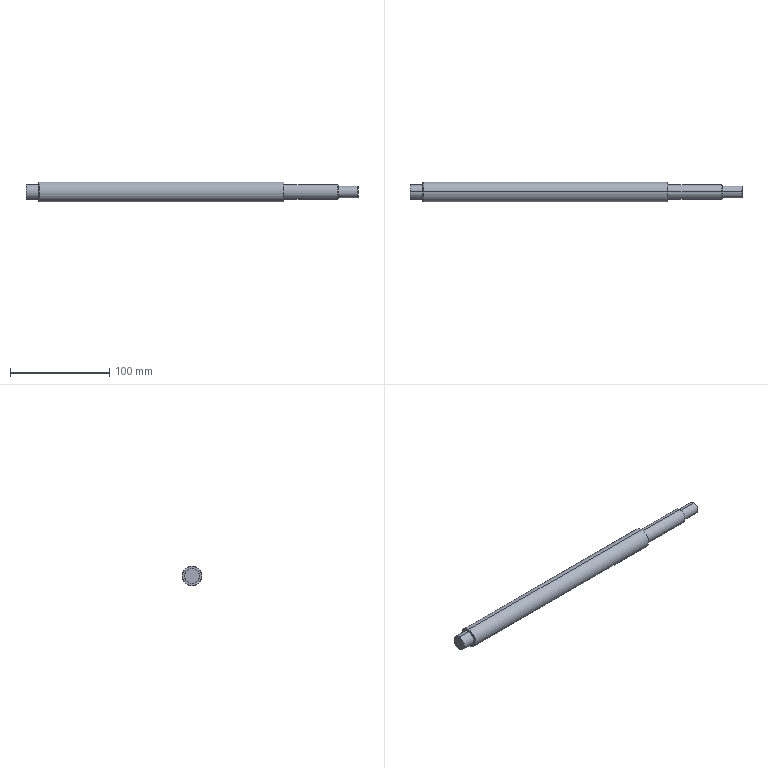Part | NX | features BREP 1 | 1 solid | 27 faces | box 335 x 20 x 20 mm | volume 91863 mm3 | cylinder 8 | torus 8 | cone 6 | plane 5 | commonest cylinder face diameters 15 x4 12 x2 20 x2
STEP:
#1=CARTESIAN_POINT('',(334.5,0.,6.));
#2=VERTEX_POINT('',#1);
#3=CARTESIAN_POINT('',(335.,0.,5.5));
#4=VERTEX_POINT('',#3);
#5=CARTESIAN_POINT('',(335.,0.,5.5));
#6=DIRECTION('',(-0.7071,0.,0.7071));
#7=VECTOR('',#6,1000.);
#8=LINE('',#5,#7);
#9=EDGE_CURVE('',#2,#4,#8,.F.);
#10=ORIENTED_EDGE('',*,*,#9,.T.);
#11=CARTESIAN_POINT('',(335.,0.,-5.5));
#12=VERTEX_POINT('',#11);
#13=CARTESIAN_POINT('',(335.,0.,0.));
#14=DIRECTION('',(1.,0.,0.));
#15=DIRECTION('',(0.,0.,-1.));
#16=AXIS2_PLACEMENT_3D('',#13,#14,#15);
#17=CIRCLE('',#16,5.5);
#18=EDGE_CURVE('',#12,#4,#17,.T.);
#19=ORIENTED_EDGE('',*,*,#18,.F.);
#20=CARTESIAN_POINT('',(334.5,0.,-6.));
#21=VERTEX_POINT('',#20);
#22=CARTESIAN_POINT('',(335.,0.,-5.5));
#23=DIRECTION('',(-0.7071,0.,-0.7071));
#24=VECTOR('',#23,1000.);
#25=LINE('',#22,#24);
#26=EDGE_CURVE('',#21,#12,#25,.F.);
#27=ORIENTED_EDGE('',*,*,#26,.F.);
#28=CARTESIAN_POINT('',(334.5,0.,0.));
#29=DIRECTION('',(1.,0.,0.));
#30=DIRECTION('',(0.,0.,-1.));
#31=AXIS2_PLACEMENT_3D('',#28,#29,#30);
#32=CIRCLE('',#31,6.);
#33=EDGE_CURVE('',#21,#2,#32,.T.);
#34=ORIENTED_EDGE('',*,*,#33,.T.);
#35=EDGE_LOOP('',(#10,#19,#27,#34));
#36=FACE_BOUND('',#35,.T.);
#37=CARTESIAN_POINT('',(334.75,0.,0.));
#38=DIRECTION('',(-1.,0.,0.));
#39=DIRECTION('',(0.,0.,1.));
#40=AXIS2_PLACEMENT_3D('',#37,#38,#39);
#41=CONICAL_SURFACE('',#40,5.75,0.7854);
#42=ADVANCED_FACE('',(#36),#41,.T.);
#43=CARTESIAN_POINT('',(315.,0.,6.));
#44=VERTEX_POINT('',#43);
#45=CARTESIAN_POINT('',(334.5,0.,6.));
#46=DIRECTION('',(-1.,0.,0.));
#47=VECTOR('',#46,1000.);
#48=LINE('',#45,#47);
#49=EDGE_CURVE('',#44,#2,#48,.F.);
#50=ORIENTED_EDGE('',*,*,#49,.T.);
#51=ORIENTED_EDGE('',*,*,#33,.F.);
#52=CARTESIAN_POINT('',(315.,0.,-6.));
#53=VERTEX_POINT('',#52);
#54=CARTESIAN_POINT('',(334.5,0.,-6.));
#55=DIRECTION('',(-1.,0.,0.));
#56=VECTOR('',#55,1000.);
#57=LINE('',#54,#56);
#58=EDGE_CURVE('',#53,#21,#57,.F.);
#59=ORIENTED_EDGE('',*,*,#58,.F.);
#60=CARTESIAN_POINT('',(315.,0.,0.));
#61=DIRECTION('',(-1.,0.,0.));
#62=DIRECTION('',(0.,0.,1.));
#63=AXIS2_PLACEMENT_3D('',#60,#61,#62);
#64=CIRCLE('',#63,6.);
#65=EDGE_CURVE('',#44,#53,#64,.T.);
#66=ORIENTED_EDGE('',*,*,#65,.F.);
#67=EDGE_LOOP('',(#50,#51,#59,#66));
#68=FACE_BOUND('',#67,.T.);
#69=CARTESIAN_POINT('',(335.,0.,0.));
#70=DIRECTION('',(-1.,0.,0.));
#71=DIRECTION('',(0.,0.,-1.));
#72=AXIS2_PLACEMENT_3D('',#69,#70,#71);
#73=CYLINDRICAL_SURFACE('',#72,6.);
#74=ADVANCED_FACE('',(#68),#73,.T.);
#75=CARTESIAN_POINT('',(315.,0.,7.));
#76=VERTEX_POINT('',#75);
#77=CARTESIAN_POINT('',(315.,0.,-7.));
#78=VERTEX_POINT('',#77);
#79=CARTESIAN_POINT('',(315.,0.,0.));
#80=DIRECTION('',(1.,0.,0.));
#81=DIRECTION('',(0.,0.,1.));
#82=AXIS2_PLACEMENT_3D('',#79,#80,#81);
#83=CIRCLE('',#82,7.);
#84=EDGE_CURVE('',#76,#78,#83,.T.);
#85=ORIENTED_EDGE('',*,*,#84,.T.);
#86=CARTESIAN_POINT('',(315.,0.,0.));
#87=DIRECTION('',(1.,0.,0.));
#88=DIRECTION('',(0.,0.,-1.));
#89=AXIS2_PLACEMENT_3D('',#86,#87,#88);
#90=CIRCLE('',#89,7.);
#91=EDGE_CURVE('',#78,#76,#90,.T.);
#92=ORIENTED_EDGE('',*,*,#91,.T.);
#93=EDGE_LOOP('',(#85,#92));
#94=FACE_BOUND('',#93,.T.);
#95=ORIENTED_EDGE('',*,*,#65,.T.);
#96=CARTESIAN_POINT('',(315.,0.,0.));
#97=DIRECTION('',(-1.,0.,0.));
#98=DIRECTION('',(0.,0.,-1.));
#99=AXIS2_PLACEMENT_3D('',#96,#97,#98);
#100=CIRCLE('',#99,6.);
#101=EDGE_CURVE('',#53,#44,#100,.T.);
#102=ORIENTED_EDGE('',*,*,#101,.T.);
#103=EDGE_LOOP('',(#95,#102));
#104=FACE_BOUND('',#103,.T.);
#105=CARTESIAN_POINT('',(315.,7.,0.));
#106=DIRECTION('',(-1.,0.,0.));
#107=DIRECTION('',(0.,0.,1.));
#108=AXIS2_PLACEMENT_3D('',#105,#106,#107);
#109=PLANE('',#108);
#110=ADVANCED_FACE('',(#94,#104),#109,.F.);
#111=CARTESIAN_POINT('',(314.5,0.,7.5));
#112=VERTEX_POINT('',#111);
#113=CARTESIAN_POINT('',(315.,0.,7.));
#114=DIRECTION('',(-0.7071,0.,0.7071));
#115=VECTOR('',#114,1000.);
#116=LINE('',#113,#115);
#117=EDGE_CURVE('',#112,#76,#116,.F.);
#118=ORIENTED_EDGE('',*,*,#117,.T.);
#119=ORIENTED_EDGE('',*,*,#91,.F.);
#120=CARTESIAN_POINT('',(314.5,0.,-7.5));
#121=VERTEX_POINT('',#120);
#122=CARTESIAN_POINT('',(315.,0.,-7.));
#123=DIRECTION('',(-0.7071,0.,-0.7071));
#124=VECTOR('',#123,1000.);
#125=LINE('',#122,#124);
#126=EDGE_CURVE('',#121,#78,#125,.F.);
#127=ORIENTED_EDGE('',*,*,#126,.F.);
#128=CARTESIAN_POINT('',(314.5,0.,0.));
#129=DIRECTION('',(1.,0.,0.));
#130=DIRECTION('',(0.,0.,-1.));
#131=AXIS2_PLACEMENT_3D('',#128,#129,#130);
#132=CIRCLE('',#131,7.5);
#133=EDGE_CURVE('',#121,#112,#132,.T.);
#134=ORIENTED_EDGE('',*,*,#133,.T.);
#135=EDGE_LOOP('',(#118,#119,#127,#134));
#136=FACE_BOUND('',#135,.T.);
#137=CARTESIAN_POINT('',(314.75,0.,0.));
#138=DIRECTION('',(-1.,0.,0.));
#139=DIRECTION('',(0.,0.,1.));
#140=AXIS2_PLACEMENT_3D('',#137,#138,#139);
#141=CONICAL_SURFACE('',#140,7.25,0.7854);
#142=ADVANCED_FACE('',(#136),#141,.T.);
#143=CARTESIAN_POINT('',(260.1,0.,7.5));
#144=VERTEX_POINT('',#143);
#145=CARTESIAN_POINT('',(314.5,0.,7.5));
#146=DIRECTION('',(-1.,0.,0.));
#147=VECTOR('',#146,1000.);
#148=LINE('',#145,#147);
#149=EDGE_CURVE('',#144,#112,#148,.F.);
#150=ORIENTED_EDGE('',*,*,#149,.T.);
#151=ORIENTED_EDGE('',*,*,#133,.F.);
#152=CARTESIAN_POINT('',(260.1,0.,-7.5));
#153=VERTEX_POINT('',#152);
#154=CARTESIAN_POINT('',(314.5,0.,-7.5));
#155=DIRECTION('',(-1.,0.,0.));
#156=VECTOR('',#155,1000.);
#157=LINE('',#154,#156);
#158=EDGE_CURVE('',#153,#121,#157,.F.);
#159=ORIENTED_EDGE('',*,*,#158,.F.);
#160=CARTESIAN_POINT('',(260.1,0.,0.));
#161=DIRECTION('',(-1.,0.,0.));
#162=DIRECTION('',(0.,0.,1.));
#163=AXIS2_PLACEMENT_3D('',#160,#161,#162);
#164=CIRCLE('',#163,7.5);
#165=EDGE_CURVE('',#144,#153,#164,.T.);
#166=ORIENTED_EDGE('',*,*,#165,.F.);
#167=EDGE_LOOP('',(#150,#151,#159,#166));
#168=FACE_BOUND('',#167,.T.);
#169=CARTESIAN_POINT('',(335.,0.,0.));
#170=DIRECTION('',(-1.,0.,0.));
#171=DIRECTION('',(0.,0.,-1.));
#172=AXIS2_PLACEMENT_3D('',#169,#170,#171);
#173=CYLINDRICAL_SURFACE('',#172,7.5);
#174=ADVANCED_FACE('',(#168),#173,.T.);
#175=CARTESIAN_POINT('',(260.029,0.,-7.529));
#176=VERTEX_POINT('',#175);
#177=CARTESIAN_POINT('',(260.1,0.,-7.6));
#178=DIRECTION('',(0.,-1.,0.));
#179=DIRECTION('',(0.,0.,1.));
#180=AXIS2_PLACEMENT_3D('',#177,#178,#179);
#181=CIRCLE('',#180,0.1);
#182=EDGE_CURVE('',#153,#176,#181,.T.);
#183=ORIENTED_EDGE('',*,*,#182,.T.);
#184=CARTESIAN_POINT('',(260.029,0.,7.529));
#185=VERTEX_POINT('',#184);
#186=CARTESIAN_POINT('',(260.029,0.,0.));
#187=DIRECTION('',(1.,0.,0.));
#188=DIRECTION('',(0.,0.,-1.));
#189=AXIS2_PLACEMENT_3D('',#186,#187,#188);
#190=CIRCLE('',#189,7.529);
#191=EDGE_CURVE('',#176,#185,#190,.T.);
#192=ORIENTED_EDGE('',*,*,#191,.T.);
#193=CARTESIAN_POINT('',(260.1,0.,7.6));
#194=DIRECTION('',(0.,1.,0.));
#195=DIRECTION('',(0.,0.,-1.));
#196=AXIS2_PLACEMENT_3D('',#193,#194,#195);
#197=CIRCLE('',#196,0.1);
#198=EDGE_CURVE('',#144,#185,#197,.T.);
#199=ORIENTED_EDGE('',*,*,#198,.F.);
#200=ORIENTED_EDGE('',*,*,#165,.T.);
#201=EDGE_LOOP('',(#183,#192,#199,#200));
#202=FACE_BOUND('',#201,.T.);
#203=CARTESIAN_POINT('',(260.1,0.,0.));
#204=DIRECTION('',(1.,0.,0.));
#205=DIRECTION('',(0.,0.,-1.));
#206=AXIS2_PLACEMENT_3D('',#203,#204,#205);
#207=TOROIDAL_SURFACE('',#206,7.6,0.1);
#208=ADVANCED_FACE('',(#202),#207,.F.);
#209=ORIENTED_EDGE('',*,*,#198,.T.);
#210=CARTESIAN_POINT('',(260.029,0.,0.));
#211=DIRECTION('',(1.,0.,0.));
#212=DIRECTION('',(0.,0.,1.));
#213=AXIS2_PLACEMENT_3D('',#210,#211,#212);
#214=CIRCLE('',#213,7.529);
#215=EDGE_CURVE('',#185,#176,#214,.T.);
#216=ORIENTED_EDGE('',*,*,#215,.T.);
#217=ORIENTED_EDGE('',*,*,#182,.F.);
#218=CARTESIAN_POINT('',(260.1,0.,0.));
#219=DIRECTION('',(-1.,0.,0.));
#220=DIRECTION('',(0.,0.,-1.));
#221=AXIS2_PLACEMENT_3D('',#218,#219,#220);
#222=CIRCLE('',#221,7.5);
#223=EDGE_CURVE('',#153,#144,#222,.T.);
#224=ORIENTED_EDGE('',*,*,#223,.T.);
#225=EDGE_LOOP('',(#209,#216,#217,#224));
#226=FACE_BOUND('',#225,.T.);
#227=CARTESIAN_POINT('',(260.1,0.,0.));
#228=DIRECTION('',(1.,0.,0.));
#229=DIRECTION('',(0.,0.,-1.));
#230=AXIS2_PLACEMENT_3D('',#227,#228,#229);
#231=TOROIDAL_SURFACE('',#230,7.6,0.1);
#232=ADVANCED_FACE('',(#226),#231,.F.);
#233=ORIENTED_EDGE('',*,*,#158,.T.);
#234=CARTESIAN_POINT('',(314.5,0.,0.));
#235=DIRECTION('',(1.,0.,0.));
#236=DIRECTION('',(0.,0.,1.));
#237=AXIS2_PLACEMENT_3D('',#234,#235,#236);
#238=CIRCLE('',#237,7.5);
#239=EDGE_CURVE('',#112,#121,#238,.T.);
#240=ORIENTED_EDGE('',*,*,#239,.F.);
#241=ORIENTED_EDGE('',*,*,#149,.F.);
#242=ORIENTED_EDGE('',*,*,#223,.F.);
#243=EDGE_LOOP('',(#233,#240,#241,#242));
#244=FACE_BOUND('',#243,.T.);
#245=CARTESIAN_POINT('',(335.,0.,0.));
#246=DIRECTION('',(-1.,0.,0.));
#247=DIRECTION('',(0.,0.,-1.));
#248=AXIS2_PLACEMENT_3D('',#245,#246,#247);
#249=CYLINDRICAL_SURFACE('',#248,7.5);
#250=ADVANCED_FACE('',(#244),#249,.T.);
#251=ORIENTED_EDGE('',*,*,#126,.T.);
#252=ORIENTED_EDGE('',*,*,#84,.F.);
#253=ORIENTED_EDGE('',*,*,#117,.F.);
#254=ORIENTED_EDGE('',*,*,#239,.T.);
#255=EDGE_LOOP('',(#251,#252,#253,#254));
#256=FACE_BOUND('',#255,.T.);
#257=CARTESIAN_POINT('',(314.75,0.,0.));
#258=DIRECTION('',(-1.,0.,0.));
#259=DIRECTION('',(0.,0.,1.));
#260=AXIS2_PLACEMENT_3D('',#257,#258,#259);
#261=CONICAL_SURFACE('',#260,7.25,0.7854);
#262=ADVANCED_FACE('',(#256),#261,.T.);
#263=CARTESIAN_POINT('',(260.,0.,-7.6));
#264=VERTEX_POINT('',#263);
#265=CARTESIAN_POINT('',(260.1,0.,-7.6));
#266=DIRECTION('',(0.,-1.,0.));
#267=DIRECTION('',(-0.7071,0.,0.7071));
#268=AXIS2_PLACEMENT_3D('',#265,#266,#267);
#269=CIRCLE('',#268,0.1);
#270=EDGE_CURVE('',#176,#264,#269,.T.);
#271=ORIENTED_EDGE('',*,*,#270,.F.);
#272=ORIENTED_EDGE('',*,*,#215,.F.);
#273=CARTESIAN_POINT('',(260.,0.,7.6));
#274=VERTEX_POINT('',#273);
#275=CARTESIAN_POINT('',(260.1,0.,7.6));
#276=DIRECTION('',(0.,1.,0.));
#277=DIRECTION('',(-0.7071,0.,-0.7071));
#278=AXIS2_PLACEMENT_3D('',#275,#276,#277);
#279=CIRCLE('',#278,0.1);
#280=EDGE_CURVE('',#185,#274,#279,.T.);
#281=ORIENTED_EDGE('',*,*,#280,.T.);
#282=CARTESIAN_POINT('',(260.,0.,0.));
#283=DIRECTION('',(-1.,0.,0.));
#284=DIRECTION('',(0.,0.,-1.));
#285=AXIS2_PLACEMENT_3D('',#282,#283,#284);
#286=CIRCLE('',#285,7.6);
#287=EDGE_CURVE('',#264,#274,#286,.T.);
#288=ORIENTED_EDGE('',*,*,#287,.F.);
#289=EDGE_LOOP('',(#271,#272,#281,#288));
#290=FACE_BOUND('',#289,.T.);
#291=CARTESIAN_POINT('',(260.1,0.,0.));
#292=DIRECTION('',(1.,0.,0.));
#293=DIRECTION('',(0.,0.,-1.));
#294=AXIS2_PLACEMENT_3D('',#291,#292,#293);
#295=TOROIDAL_SURFACE('',#294,7.6,0.1);
#296=ADVANCED_FACE('',(#290),#295,.F.);
#297=CARTESIAN_POINT('',(260.,0.,10.));
#298=VERTEX_POINT('',#297);
#299=CARTESIAN_POINT('',(260.,0.,-10.));
#300=VERTEX_POINT('',#299);
#301=CARTESIAN_POINT('',(260.,0.,0.));
#302=DIRECTION('',(1.,0.,0.));
#303=DIRECTION('',(0.,0.,1.));
#304=AXIS2_PLACEMENT_3D('',#301,#302,#303);
#305=CIRCLE('',#304,10.);
#306=EDGE_CURVE('',#298,#300,#305,.T.);
#307=ORIENTED_EDGE('',*,*,#306,.T.);
#308=CARTESIAN_POINT('',(260.,0.,0.));
#309=DIRECTION('',(1.,0.,0.));
#310=DIRECTION('',(0.,0.,-1.));
#311=AXIS2_PLACEMENT_3D('',#308,#309,#310);
#312=CIRCLE('',#311,10.);
#313=EDGE_CURVE('',#300,#298,#312,.T.);
#314=ORIENTED_EDGE('',*,*,#313,.T.);
#315=EDGE_LOOP('',(#307,#314));
#316=FACE_BOUND('',#315,.T.);
#317=CARTESIAN_POINT('',(260.,0.,0.));
#318=DIRECTION('',(-1.,0.,0.));
#319=DIRECTION('',(0.,0.,1.));
#320=AXIS2_PLACEMENT_3D('',#317,#318,#319);
#321=CIRCLE('',#320,7.6);
#322=EDGE_CURVE('',#274,#264,#321,.T.);
#323=ORIENTED_EDGE('',*,*,#322,.T.);
#324=ORIENTED_EDGE('',*,*,#287,.T.);
#325=EDGE_LOOP('',(#323,#324));
#326=FACE_BOUND('',#325,.T.);
#327=CARTESIAN_POINT('',(260.,10.,0.));
#328=DIRECTION('',(-1.,0.,0.));
#329=DIRECTION('',(0.,0.,1.));
#330=AXIS2_PLACEMENT_3D('',#327,#328,#329);
#331=PLANE('',#330);
#332=ADVANCED_FACE('',(#316,#326),#331,.F.);
#333=CARTESIAN_POINT('',(13.3,0.,10.));
#334=VERTEX_POINT('',#333);
#335=CARTESIAN_POINT('',(260.,0.,10.));
#336=DIRECTION('',(-1.,0.,0.));
#337=VECTOR('',#336,1000.);
#338=LINE('',#335,#337);
#339=EDGE_CURVE('',#334,#298,#338,.F.);
#340=ORIENTED_EDGE('',*,*,#339,.T.);
#341=ORIENTED_EDGE('',*,*,#313,.F.);
#342=CARTESIAN_POINT('',(13.3,0.,-10.));
#343=VERTEX_POINT('',#342);
#344=CARTESIAN_POINT('',(260.,0.,-10.));
#345=DIRECTION('',(-1.,0.,0.));
#346=VECTOR('',#345,1000.);
#347=LINE('',#344,#346);
#348=EDGE_CURVE('',#343,#300,#347,.F.);
#349=ORIENTED_EDGE('',*,*,#348,.F.);
#350=CARTESIAN_POINT('',(13.3,0.,0.));
#351=DIRECTION('',(-1.,0.,0.));
#352=DIRECTION('',(0.,0.,1.));
#353=AXIS2_PLACEMENT_3D('',#350,#351,#352);
#354=CIRCLE('',#353,10.);
#355=EDGE_CURVE('',#334,#343,#354,.T.);
#356=ORIENTED_EDGE('',*,*,#355,.F.);
#357=EDGE_LOOP('',(#340,#341,#349,#356));
#358=FACE_BOUND('',#357,.T.);
#359=CARTESIAN_POINT('',(335.,0.,0.));
#360=DIRECTION('',(-1.,0.,0.));
#361=DIRECTION('',(0.,0.,-1.));
#362=AXIS2_PLACEMENT_3D('',#359,#360,#361);
#363=CYLINDRICAL_SURFACE('',#362,10.);
#364=ADVANCED_FACE('',(#358),#363,.T.);
#365=CARTESIAN_POINT('',(13.,0.,-9.7));
#366=VERTEX_POINT('',#365);
#367=CARTESIAN_POINT('',(13.,0.,-9.7));
#368=DIRECTION('',(0.7071,0.,-0.7071));
#369=VECTOR('',#368,1000.);
#370=LINE('',#367,#369);
#371=EDGE_CURVE('',#366,#343,#370,.T.);
#372=ORIENTED_EDGE('',*,*,#371,.F.);
#373=CARTESIAN_POINT('',(13.,0.,9.7));
#374=VERTEX_POINT('',#373);
#375=CARTESIAN_POINT('',(13.,0.,0.));
#376=DIRECTION('',(-1.,0.,0.));
#377=DIRECTION('',(0.,0.,1.));
#378=AXIS2_PLACEMENT_3D('',#375,#376,#377);
#379=CIRCLE('',#378,9.7);
#380=EDGE_CURVE('',#374,#366,#379,.T.);
#381=ORIENTED_EDGE('',*,*,#380,.F.);
#382=CARTESIAN_POINT('',(13.,0.,9.7));
#383=DIRECTION('',(0.7071,0.,0.7071));
#384=VECTOR('',#383,1000.);
#385=LINE('',#382,#384);
#386=EDGE_CURVE('',#374,#334,#385,.T.);
#387=ORIENTED_EDGE('',*,*,#386,.T.);
#388=ORIENTED_EDGE('',*,*,#355,.T.);
#389=EDGE_LOOP('',(#372,#381,#387,#388));
#390=FACE_BOUND('',#389,.T.);
#391=CARTESIAN_POINT('',(13.15,0.,0.));
#392=DIRECTION('',(1.,0.,0.));
#393=DIRECTION('',(0.,0.,-1.));
#394=AXIS2_PLACEMENT_3D('',#391,#392,#393);
#395=CONICAL_SURFACE('',#394,9.85,0.7854);
#396=ADVANCED_FACE('',(#390),#395,.T.);
#397=ORIENTED_EDGE('',*,*,#386,.F.);
#398=CARTESIAN_POINT('',(13.,0.,0.));
#399=DIRECTION('',(-1.,0.,0.));
#400=DIRECTION('',(0.,0.,-1.));
#401=AXIS2_PLACEMENT_3D('',#398,#399,#400);
#402=CIRCLE('',#401,9.7);
#403=EDGE_CURVE('',#366,#374,#402,.T.);
#404=ORIENTED_EDGE('',*,*,#403,.F.);
#405=ORIENTED_EDGE('',*,*,#371,.T.);
#406=CARTESIAN_POINT('',(13.3,0.,0.));
#407=DIRECTION('',(-1.,0.,0.));
#408=DIRECTION('',(0.,0.,-1.));
#409=AXIS2_PLACEMENT_3D('',#406,#407,#408);
#410=CIRCLE('',#409,10.);
#411=EDGE_CURVE('',#343,#334,#410,.T.);
#412=ORIENTED_EDGE('',*,*,#411,.T.);
#413=EDGE_LOOP('',(#397,#404,#405,#412));
#414=FACE_BOUND('',#413,.T.);
#415=CARTESIAN_POINT('',(13.15,0.,0.));
#416=DIRECTION('',(1.,0.,0.));
#417=DIRECTION('',(0.,0.,-1.));
#418=AXIS2_PLACEMENT_3D('',#415,#416,#417);
#419=CONICAL_SURFACE('',#418,9.85,0.7854);
#420=ADVANCED_FACE('',(#414),#419,.T.);
#421=ORIENTED_EDGE('',*,*,#348,.T.);
#422=ORIENTED_EDGE('',*,*,#306,.F.);
#423=ORIENTED_EDGE('',*,*,#339,.F.);
#424=ORIENTED_EDGE('',*,*,#411,.F.);
#425=EDGE_LOOP('',(#421,#422,#423,#424));
#426=FACE_BOUND('',#425,.T.);
#427=CARTESIAN_POINT('',(335.,0.,0.));
#428=DIRECTION('',(-1.,0.,0.));
#429=DIRECTION('',(0.,0.,-1.));
#430=AXIS2_PLACEMENT_3D('',#427,#428,#429);
#431=CYLINDRICAL_SURFACE('',#430,10.);
#432=ADVANCED_FACE('',(#426),#431,.T.);
#433=ORIENTED_EDGE('',*,*,#380,.T.);
#434=ORIENTED_EDGE('',*,*,#403,.T.);
#435=EDGE_LOOP('',(#433,#434));
#436=FACE_BOUND('',#435,.T.);
#437=CARTESIAN_POINT('',(13.,0.,7.6));
#438=VERTEX_POINT('',#437);
#439=CARTESIAN_POINT('',(13.,0.,-7.6));
#440=VERTEX_POINT('',#439);
#441=CARTESIAN_POINT('',(13.,0.,0.));
#442=DIRECTION('',(1.,0.,0.));
#443=DIRECTION('',(0.,0.,1.));
#444=AXIS2_PLACEMENT_3D('',#441,#442,#443);
#445=CIRCLE('',#444,7.6);
#446=EDGE_CURVE('',#438,#440,#445,.T.);
#447=ORIENTED_EDGE('',*,*,#446,.T.);
#448=CARTESIAN_POINT('',(13.,0.,0.));
#449=DIRECTION('',(1.,0.,0.));
#450=DIRECTION('',(0.,0.,-1.));
#451=AXIS2_PLACEMENT_3D('',#448,#449,#450);
#452=CIRCLE('',#451,7.6);
#453=EDGE_CURVE('',#440,#438,#452,.T.);
#454=ORIENTED_EDGE('',*,*,#453,.T.);
#455=EDGE_LOOP('',(#447,#454));
#456=FACE_BOUND('',#455,.T.);
#457=CARTESIAN_POINT('',(13.,7.6,0.));
#458=DIRECTION('',(1.,0.,0.));
#459=DIRECTION('',(0.,1.,0.));
#460=AXIS2_PLACEMENT_3D('',#457,#458,#459);
#461=PLANE('',#460);
#462=ADVANCED_FACE('',(#436,#456),#461,.F.);
#463=CARTESIAN_POINT('',(12.971,0.,-7.529));
#464=VERTEX_POINT('',#463);
#465=CARTESIAN_POINT('',(12.9,0.,-7.6));
#466=DIRECTION('',(0.,-1.,0.));
#467=DIRECTION('',(1.,0.,0.));
#468=AXIS2_PLACEMENT_3D('',#465,#466,#467);
#469=CIRCLE('',#468,0.1);
#470=EDGE_CURVE('',#440,#464,#469,.T.);
#471=ORIENTED_EDGE('',*,*,#470,.T.);
#472=CARTESIAN_POINT('',(12.971,0.,7.529));
#473=VERTEX_POINT('',#472);
#474=CARTESIAN_POINT('',(12.971,0.,0.));
#475=DIRECTION('',(1.,0.,0.));
#476=DIRECTION('',(0.,0.,-1.));
#477=AXIS2_PLACEMENT_3D('',#474,#475,#476);
#478=CIRCLE('',#477,7.529);
#479=EDGE_CURVE('',#464,#473,#478,.T.);
#480=ORIENTED_EDGE('',*,*,#479,.T.);
#481=CARTESIAN_POINT('',(12.9,0.,7.6));
#482=DIRECTION('',(0.,1.,0.));
#483=DIRECTION('',(1.,0.,0.));
#484=AXIS2_PLACEMENT_3D('',#481,#482,#483);
#485=CIRCLE('',#484,0.1);
#486=EDGE_CURVE('',#438,#473,#485,.T.);
#487=ORIENTED_EDGE('',*,*,#486,.F.);
#488=ORIENTED_EDGE('',*,*,#453,.F.);
#489=EDGE_LOOP('',(#471,#480,#487,#488));
#490=FACE_BOUND('',#489,.T.);
#491=CARTESIAN_POINT('',(12.9,0.,0.));
#492=DIRECTION('',(1.,0.,0.));
#493=DIRECTION('',(0.,0.,-1.));
#494=AXIS2_PLACEMENT_3D('',#491,#492,#493);
#495=TOROIDAL_SURFACE('',#494,7.6,0.1);
#496=ADVANCED_FACE('',(#490),#495,.F.);
#497=ORIENTED_EDGE('',*,*,#486,.T.);
#498=CARTESIAN_POINT('',(12.971,0.,0.));
#499=DIRECTION('',(1.,0.,0.));
#500=DIRECTION('',(0.,0.,1.));
#501=AXIS2_PLACEMENT_3D('',#498,#499,#500);
#502=CIRCLE('',#501,7.529);
#503=EDGE_CURVE('',#473,#464,#502,.T.);
#504=ORIENTED_EDGE('',*,*,#503,.T.);
#505=ORIENTED_EDGE('',*,*,#470,.F.);
#506=ORIENTED_EDGE('',*,*,#446,.F.);
#507=EDGE_LOOP('',(#497,#504,#505,#506));
#508=FACE_BOUND('',#507,.T.);
#509=CARTESIAN_POINT('',(12.9,0.,0.));
#510=DIRECTION('',(1.,0.,0.));
#511=DIRECTION('',(0.,0.,-1.));
#512=AXIS2_PLACEMENT_3D('',#509,#510,#511);
#513=TOROIDAL_SURFACE('',#512,7.6,0.1);
#514=ADVANCED_FACE('',(#508),#513,.F.);
#515=CARTESIAN_POINT('',(12.9,0.,-7.5));
#516=VERTEX_POINT('',#515);
#517=CARTESIAN_POINT('',(12.9,0.,-7.6));
#518=DIRECTION('',(0.,-1.,0.));
#519=DIRECTION('',(0.7071,0.,0.7071));
#520=AXIS2_PLACEMENT_3D('',#517,#518,#519);
#521=CIRCLE('',#520,0.1);
#522=EDGE_CURVE('',#464,#516,#521,.T.);
#523=ORIENTED_EDGE('',*,*,#522,.F.);
#524=ORIENTED_EDGE('',*,*,#503,.F.);
#525=CARTESIAN_POINT('',(12.9,0.,7.5));
#526=VERTEX_POINT('',#525);
#527=CARTESIAN_POINT('',(12.9,0.,7.6));
#528=DIRECTION('',(0.,1.,0.));
#529=DIRECTION('',(0.7071,0.,-0.7071));
#530=AXIS2_PLACEMENT_3D('',#527,#528,#529);
#531=CIRCLE('',#530,0.1);
#532=EDGE_CURVE('',#473,#526,#531,.T.);
#533=ORIENTED_EDGE('',*,*,#532,.T.);
#534=CARTESIAN_POINT('',(12.9,0.,0.));
#535=DIRECTION('',(1.,0.,0.));
#536=DIRECTION('',(0.,0.,1.));
#537=AXIS2_PLACEMENT_3D('',#534,#535,#536);
#538=CIRCLE('',#537,7.5);
#539=EDGE_CURVE('',#526,#516,#538,.T.);
#540=ORIENTED_EDGE('',*,*,#539,.T.);
#541=EDGE_LOOP('',(#523,#524,#533,#540));
#542=FACE_BOUND('',#541,.T.);
#543=CARTESIAN_POINT('',(12.9,0.,0.));
#544=DIRECTION('',(1.,0.,0.));
#545=DIRECTION('',(0.,0.,-1.));
#546=AXIS2_PLACEMENT_3D('',#543,#544,#545);
#547=TOROIDAL_SURFACE('',#546,7.6,0.1);
#548=ADVANCED_FACE('',(#542),#547,.F.);
#549=CARTESIAN_POINT('',(0.,0.,-7.5));
#550=VERTEX_POINT('',#549);
#551=CARTESIAN_POINT('',(12.9,0.,-7.5));
#552=DIRECTION('',(-1.,0.,0.));
#553=VECTOR('',#552,1000.);
#554=LINE('',#551,#553);
#555=EDGE_CURVE('',#516,#550,#554,.T.);
#556=ORIENTED_EDGE('',*,*,#555,.F.);
#557=ORIENTED_EDGE('',*,*,#539,.F.);
#558=CARTESIAN_POINT('',(0.,0.,7.5));
#559=VERTEX_POINT('',#558);
#560=CARTESIAN_POINT('',(12.9,0.,7.5));
#561=DIRECTION('',(-1.,0.,0.));
#562=VECTOR('',#561,1000.);
#563=LINE('',#560,#562);
#564=EDGE_CURVE('',#526,#559,#563,.T.);
#565=ORIENTED_EDGE('',*,*,#564,.T.);
#566=CARTESIAN_POINT('',(0.,0.,0.));
#567=DIRECTION('',(-1.,0.,0.));
#568=DIRECTION('',(0.,0.,-1.));
#569=AXIS2_PLACEMENT_3D('',#566,#567,#568);
#570=CIRCLE('',#569,7.5);
#571=EDGE_CURVE('',#550,#559,#570,.T.);
#572=ORIENTED_EDGE('',*,*,#571,.F.);
#573=EDGE_LOOP('',(#556,#557,#565,#572));
#574=FACE_BOUND('',#573,.T.);
#575=CARTESIAN_POINT('',(335.,0.,0.));
#576=DIRECTION('',(-1.,0.,0.));
#577=DIRECTION('',(0.,0.,-1.));
#578=AXIS2_PLACEMENT_3D('',#575,#576,#577);
#579=CYLINDRICAL_SURFACE('',#578,7.5);
#580=ADVANCED_FACE('',(#574),#579,.T.);
#581=CARTESIAN_POINT('',(0.,0.,0.));
#582=DIRECTION('',(-1.,0.,0.));
#583=DIRECTION('',(0.,0.,1.));
#584=AXIS2_PLACEMENT_3D('',#581,#582,#583);
#585=CIRCLE('',#584,7.5);
#586=EDGE_CURVE('',#559,#550,#585,.T.);
#587=ORIENTED_EDGE('',*,*,#586,.T.);
#588=ORIENTED_EDGE('',*,*,#571,.T.);
#589=EDGE_LOOP('',(#587,#588));
#590=FACE_BOUND('',#589,.T.);
#591=CARTESIAN_POINT('',(0.,0.,0.));
#592=DIRECTION('',(1.,0.,0.));
#593=DIRECTION('',(0.,1.,0.));
#594=AXIS2_PLACEMENT_3D('',#591,#592,#593);
#595=PLANE('',#594);
#596=ADVANCED_FACE('',(#590),#595,.F.);
#597=ORIENTED_EDGE('',*,*,#564,.F.);
#598=CARTESIAN_POINT('',(12.9,0.,0.));
#599=DIRECTION('',(1.,0.,0.));
#600=DIRECTION('',(0.,0.,-1.));
#601=AXIS2_PLACEMENT_3D('',#598,#599,#600);
#602=CIRCLE('',#601,7.5);
#603=EDGE_CURVE('',#516,#526,#602,.T.);
#604=ORIENTED_EDGE('',*,*,#603,.F.);
#605=ORIENTED_EDGE('',*,*,#555,.T.);
#606=ORIENTED_EDGE('',*,*,#586,.F.);
#607=EDGE_LOOP('',(#597,#604,#605,#606));
#608=FACE_BOUND('',#607,.T.);
#609=CARTESIAN_POINT('',(335.,0.,0.));
#610=DIRECTION('',(-1.,0.,0.));
#611=DIRECTION('',(0.,0.,-1.));
#612=AXIS2_PLACEMENT_3D('',#609,#610,#611);
#613=CYLINDRICAL_SURFACE('',#612,7.5);
#614=ADVANCED_FACE('',(#608),#613,.T.);
#615=ORIENTED_EDGE('',*,*,#532,.F.);
#616=ORIENTED_EDGE('',*,*,#479,.F.);
#617=ORIENTED_EDGE('',*,*,#522,.T.);
#618=ORIENTED_EDGE('',*,*,#603,.T.);
#619=EDGE_LOOP('',(#615,#616,#617,#618));
#620=FACE_BOUND('',#619,.T.);
#621=CARTESIAN_POINT('',(12.9,0.,0.));
#622=DIRECTION('',(1.,0.,0.));
#623=DIRECTION('',(0.,0.,-1.));
#624=AXIS2_PLACEMENT_3D('',#621,#622,#623);
#625=TOROIDAL_SURFACE('',#624,7.6,0.1);
#626=ADVANCED_FACE('',(#620),#625,.F.);
#627=ORIENTED_EDGE('',*,*,#280,.F.);
#628=ORIENTED_EDGE('',*,*,#191,.F.);
#629=ORIENTED_EDGE('',*,*,#270,.T.);
#630=ORIENTED_EDGE('',*,*,#322,.F.);
#631=EDGE_LOOP('',(#627,#628,#629,#630));
#632=FACE_BOUND('',#631,.T.);
#633=CARTESIAN_POINT('',(260.1,0.,0.));
#634=DIRECTION('',(1.,0.,0.));
#635=DIRECTION('',(0.,0.,-1.));
#636=AXIS2_PLACEMENT_3D('',#633,#634,#635);
#637=TOROIDAL_SURFACE('',#636,7.6,0.1);
#638=ADVANCED_FACE('',(#632),#637,.F.);
#639=ORIENTED_EDGE('',*,*,#58,.T.);
#640=CARTESIAN_POINT('',(334.5,0.,0.));
#641=DIRECTION('',(1.,0.,0.));
#642=DIRECTION('',(0.,0.,1.));
#643=AXIS2_PLACEMENT_3D('',#640,#641,#642);
#644=CIRCLE('',#643,6.);
#645=EDGE_CURVE('',#2,#21,#644,.T.);
#646=ORIENTED_EDGE('',*,*,#645,.F.);
#647=ORIENTED_EDGE('',*,*,#49,.F.);
#648=ORIENTED_EDGE('',*,*,#101,.F.);
#649=EDGE_LOOP('',(#639,#646,#647,#648));
#650=FACE_BOUND('',#649,.T.);
#651=CARTESIAN_POINT('',(335.,0.,0.));
#652=DIRECTION('',(-1.,0.,0.));
#653=DIRECTION('',(0.,0.,-1.));
#654=AXIS2_PLACEMENT_3D('',#651,#652,#653);
#655=CYLINDRICAL_SURFACE('',#654,6.);
#656=ADVANCED_FACE('',(#650),#655,.T.);
#657=ORIENTED_EDGE('',*,*,#26,.T.);
#658=CARTESIAN_POINT('',(335.,0.,0.));
#659=DIRECTION('',(1.,0.,0.));
#660=DIRECTION('',(0.,0.,1.));
#661=AXIS2_PLACEMENT_3D('',#658,#659,#660);
#662=CIRCLE('',#661,5.5);
#663=EDGE_CURVE('',#4,#12,#662,.T.);
#664=ORIENTED_EDGE('',*,*,#663,.F.);
#665=ORIENTED_EDGE('',*,*,#9,.F.);
#666=ORIENTED_EDGE('',*,*,#645,.T.);
#667=EDGE_LOOP('',(#657,#664,#665,#666));
#668=FACE_BOUND('',#667,.T.);
#669=CARTESIAN_POINT('',(334.75,0.,0.));
#670=DIRECTION('',(-1.,0.,0.));
#671=DIRECTION('',(0.,0.,1.));
#672=AXIS2_PLACEMENT_3D('',#669,#670,#671);
#673=CONICAL_SURFACE('',#672,5.75,0.7854);
#674=ADVANCED_FACE('',(#668),#673,.T.);
#675=ORIENTED_EDGE('',*,*,#663,.T.);
#676=ORIENTED_EDGE('',*,*,#18,.T.);
#677=EDGE_LOOP('',(#675,#676));
#678=FACE_BOUND('',#677,.T.);
#679=CARTESIAN_POINT('',(335.,5.5,0.));
#680=DIRECTION('',(-1.,0.,0.));
#681=DIRECTION('',(0.,0.,1.));
#682=AXIS2_PLACEMENT_3D('',#679,#680,#681);
#683=PLANE('',#682);
#684=ADVANCED_FACE('',(#678),#683,.F.);
#685=CLOSED_SHELL('',(#42,#74,#110,#142,#174,#208,#232,#250,#262,#296,#332,#364,#396,#420,#432,#462,#496,#514,#548,#580,#596,#614,#626,#638,#656,#674,#684));
#686=MANIFOLD_SOLID_BREP('',#685);
#687=(LENGTH_UNIT()NAMED_UNIT(*)SI_UNIT(.MILLI.,.METRE.));
#688=UNCERTAINTY_MEASURE_WITH_UNIT(LENGTH_MEASURE(0.00001),#687,'','');
#689=(NAMED_UNIT(*)PLANE_ANGLE_UNIT()SI_UNIT($,.RADIAN.));
#690=(NAMED_UNIT(*)SI_UNIT($,.STERADIAN.)SOLID_ANGLE_UNIT());
#691=(GEOMETRIC_REPRESENTATION_CONTEXT(3)GLOBAL_UNCERTAINTY_ASSIGNED_CONTEXT((#688))GLOBAL_UNIT_ASSIGNED_CONTEXT((#687,#689,#690))REPRESENTATION_CONTEXT('',''));
#692=ADVANCED_BREP_SHAPE_REPRESENTATION('',(#686),#691);